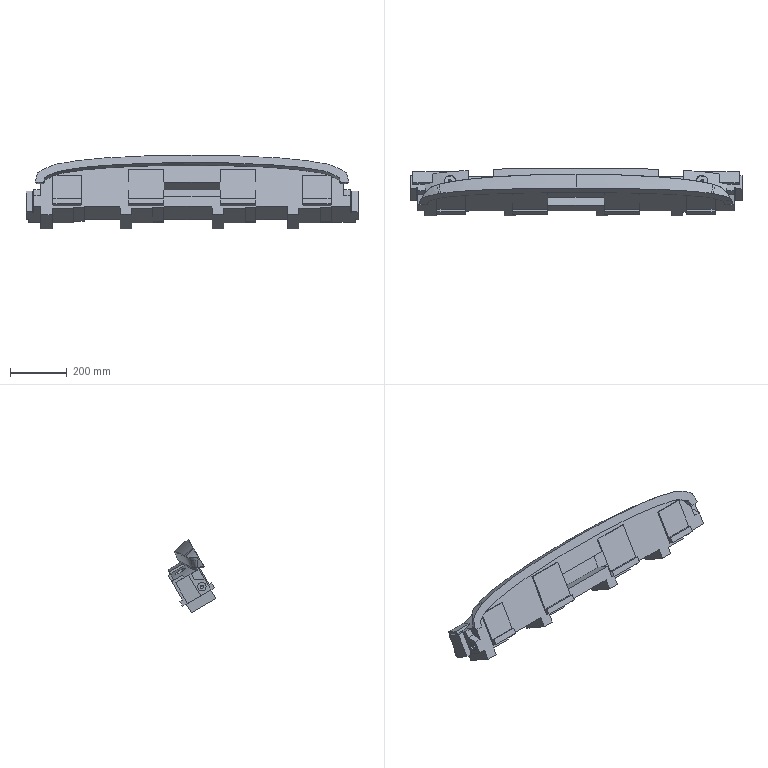Part | NX | features solid 2 | 1 solid | 220 faces | box 1170 x 168.629 x 259.562 mm | volume 16646996 mm3 | plane 143 | spline 59 | cylinder 14 | cone 4 | commonest cylinder face diameters 12 x4 60 x4 29 x2 30 x2 40 x2